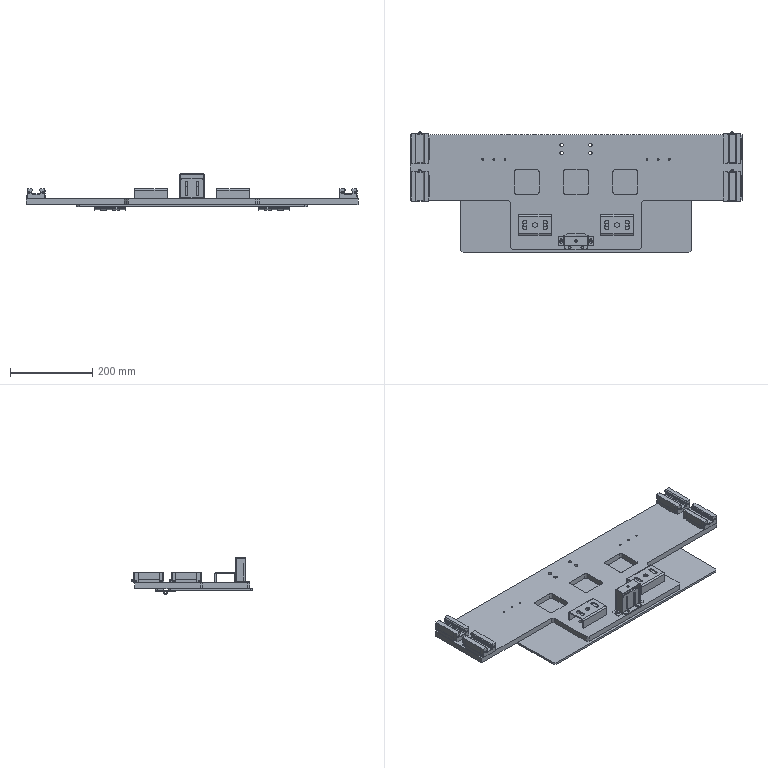Part | SolidWorks | features ReferencePattern 5, CompositeCurve 2, LocalLPattern 1, MirrorCompFeat 1 | 17 solids | 1287 faces | box 808 x 294.081 x 89.45 mm | volume 3072025 mm3 | plane 715 | cylinder 496 | cone 64 | sphere 8 | spline 4 | commonest cylinder face diameters 5 x60 6 x50 4.4 x48 2.4 x40 9 x38 0.4 x32